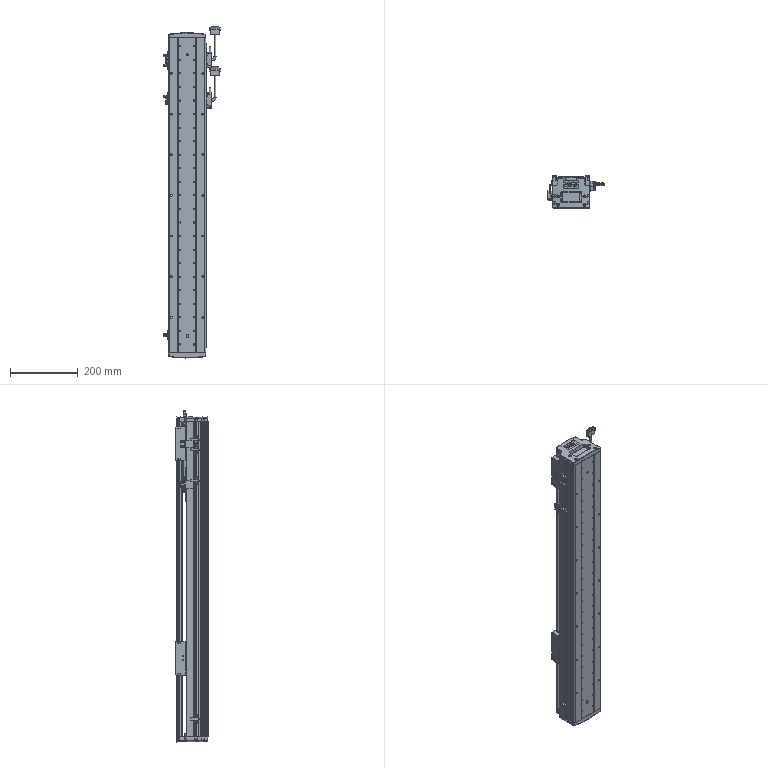Part | SolidWorks | 45 solids | 4364 faces | volume 4425715 mm3 | plane 2092 | cylinder 1758 | cone 292 | spline 222 | commonest cylinder face diameters 3.3 x232 4.5 x172 8 x160 4 x134 2 x98 4.3 x92